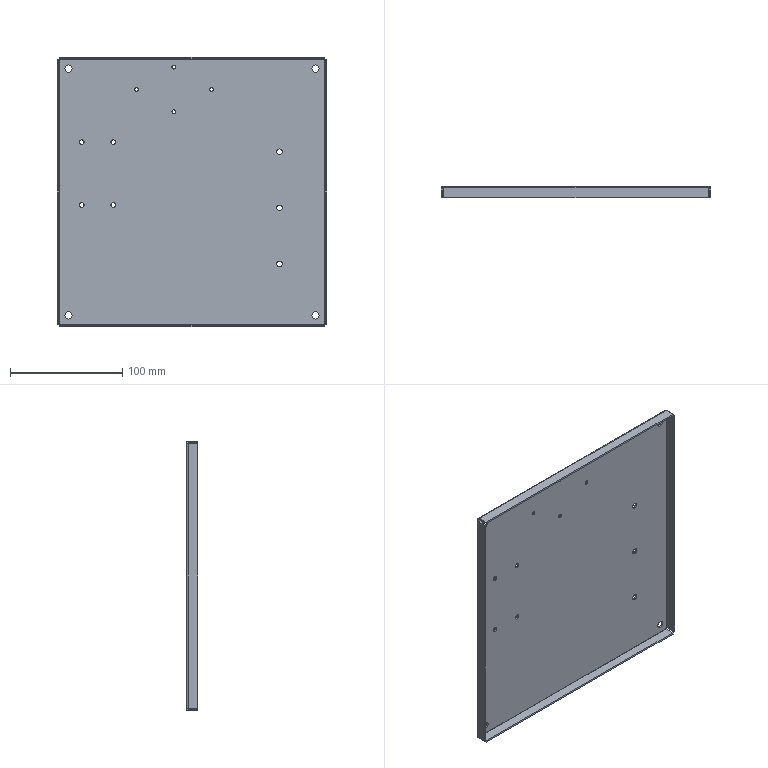Part | SolidWorks | features 3DProfileFeature 3, HoleWzd 3, EdgeFlange 1, FlatPattern 1, ICE 1, SMBaseFlange 1, SheetMetal 1 | 1 solid | 68 faces | box 240.001 x 10 x 240.001 mm | volume 97461 mm3 | cylinder 38 | plane 22 | spline 8 | commonest cylinder face diameters 3.3 x8 4.2 x8 6.4 x8 5 x6 0.2 x4 3.2 x4